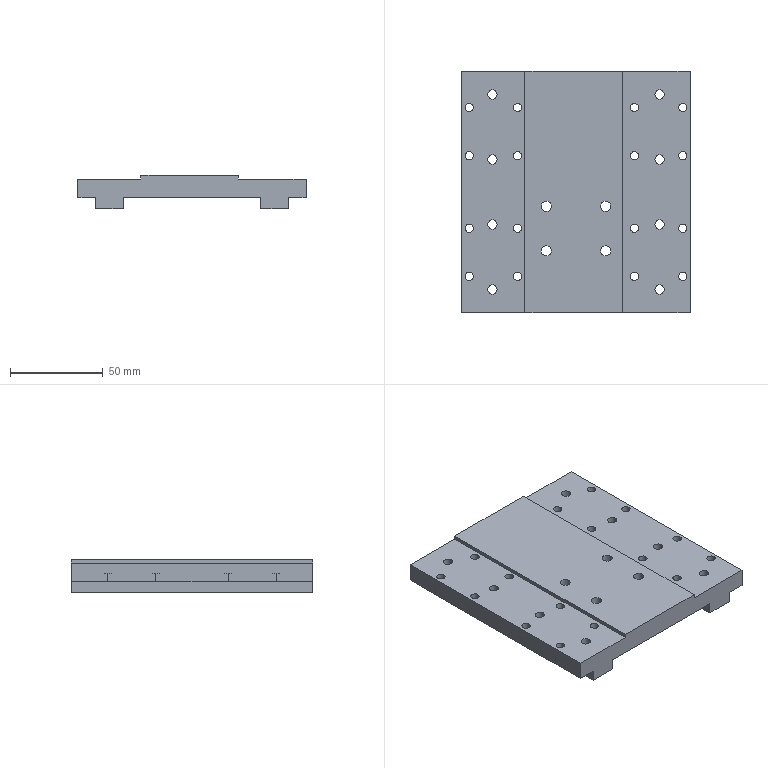Part | 1 solid | 140 faces | box 123 x 130 x 18 mm | volume 186507 mm3 | cylinder 100 | plane 40 | commonest cylinder face diameters 4.5 x32 8 x32 5 x16 5.5 x8 10 x8 6 x4